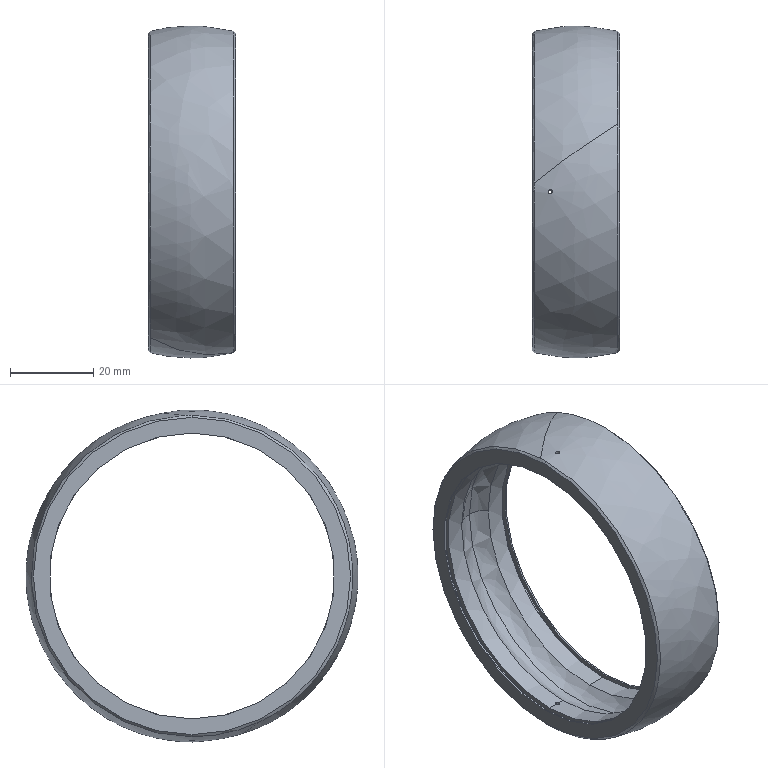Part | SolidWorks | features BaseBody 1 | 1 solid | 32 faces | box 21 x 80 x 80 mm | volume 21730 mm3 | spline 26 | plane 6
STEP:
#1=CARTESIAN_POINT('',(0.,111.35,49.2));
#2=VERTEX_POINT('',#1);
#3=CARTESIAN_POINT('',(0.,38.65,49.2));
#4=VERTEX_POINT('',#3);
#5=CARTESIAN_POINT('',(0.,75.,49.2));
#6=DIRECTION('',(-1.,0.,0.));
#7=DIRECTION('',(0.,-1.,0.));
#8=AXIS2_PLACEMENT_3D('',#5,#6,#7);
#9=CIRCLE('',#8,36.35);
#10=EDGE_CURVE('',#2,#4,#9,.T.);
#11=ORIENTED_EDGE('',*,*,#10,.F.);
#12=CARTESIAN_POINT('',(-4.535,109.445,49.2));
#13=VERTEX_POINT('',#12);
#14=CARTESIAN_POINT('',(0.,105.,49.2));
#15=DIRECTION('',(0.,0.,1.));
#16=DIRECTION('',(0.,1.,0.));
#17=AXIS2_PLACEMENT_3D('',#14,#15,#16);
#18=CIRCLE('',#17,6.35);
#19=EDGE_CURVE('',#2,#13,#18,.T.);
#20=ORIENTED_EDGE('',*,*,#19,.T.);
#21=CARTESIAN_POINT('',(-4.535,75.,14.755));
#22=VERTEX_POINT('',#21);
#23=CARTESIAN_POINT('',(-4.535,75.,49.2));
#24=DIRECTION('',(-1.,0.,0.));
#25=DIRECTION('',(0.,0.,1.));
#26=AXIS2_PLACEMENT_3D('',#23,#24,#25);
#27=CIRCLE('',#26,34.445);
#28=EDGE_CURVE('',#13,#22,#27,.T.);
#29=ORIENTED_EDGE('',*,*,#28,.T.);
#30=CARTESIAN_POINT('',(-4.535,40.555,49.2));
#31=VERTEX_POINT('',#30);
#32=CARTESIAN_POINT('',(-4.535,75.,49.2));
#33=DIRECTION('',(-1.,0.,0.));
#34=DIRECTION('',(0.,0.,1.));
#35=AXIS2_PLACEMENT_3D('',#32,#33,#34);
#36=CIRCLE('',#35,34.445);
#37=EDGE_CURVE('',#22,#31,#36,.T.);
#38=ORIENTED_EDGE('',*,*,#37,.T.);
#39=CARTESIAN_POINT('',(0.,45.,49.2));
#40=DIRECTION('',(0.,0.,-1.));
#41=DIRECTION('',(0.,-1.,0.));
#42=AXIS2_PLACEMENT_3D('',#39,#40,#41);
#43=CIRCLE('',#42,6.35);
#44=EDGE_CURVE('',#4,#31,#43,.T.);
#45=ORIENTED_EDGE('',*,*,#44,.F.);
#46=EDGE_LOOP('',(#11,#20,#29,#38,#45));
#47=FACE_OUTER_BOUND('',#46,.T.);
#48=CARTESIAN_POINT('',(0.,111.35,49.2));
#49=CARTESIAN_POINT('',(0.,111.35,-23.5));
#50=CARTESIAN_POINT('',(0.,38.65,-23.5));
#51=CARTESIAN_POINT('',(0.,38.65,49.2));
#52=CARTESIAN_POINT('',(-1.73,111.35,49.2));
#53=CARTESIAN_POINT('',(-1.73,111.35,-23.5));
#54=CARTESIAN_POINT('',(-1.73,38.65,-23.5));
#55=CARTESIAN_POINT('',(-1.73,38.65,49.2));
#56=CARTESIAN_POINT('',(-3.324,110.68,49.2));
#57=CARTESIAN_POINT('',(-3.324,110.68,-22.16));
#58=CARTESIAN_POINT('',(-3.324,39.32,-22.16));
#59=CARTESIAN_POINT('',(-3.324,39.32,49.2));
#60=CARTESIAN_POINT('',(-4.535,109.445,49.2));
#61=CARTESIAN_POINT('',(-4.535,109.445,-19.69));
#62=CARTESIAN_POINT('',(-4.535,40.555,-19.69));
#63=CARTESIAN_POINT('',(-4.535,40.555,49.2));
#64=(BOUNDED_SURFACE()B_SPLINE_SURFACE(3,3,((#48,#49,#50,#51),(#52,#53,#54,#55),(#56,#57,#58,#59),(#60,#61,#62,#63)),.UNSPECIFIED.,.F.,.F.,.F.)B_SPLINE_SURFACE_WITH_KNOTS((4,4),(4,4),(0.,1.),(0.,1.),.UNSPECIFIED.)GEOMETRIC_REPRESENTATION_ITEM()RATIONAL_B_SPLINE_SURFACE(((1.,0.3333,0.3333,1.),(0.948,0.316,0.316,0.948),(0.948,0.316,0.316,0.948),(1.,0.3333,0.3333,1.)))REPRESENTATION_ITEM('')SURFACE());
#65=ADVANCED_FACE('',(#47),#64,.T.);
#66=CARTESIAN_POINT('',(10.,75.,10.47));
#67=VERTEX_POINT('',#66);
#68=CARTESIAN_POINT('',(10.,72.909,10.527));
#69=VERTEX_POINT('',#68);
#70=CARTESIAN_POINT('',(10.,75.,49.2));
#71=DIRECTION('',(-1.,0.,0.));
#72=DIRECTION('',(0.,0.,1.));
#73=AXIS2_PLACEMENT_3D('',#70,#71,#72);
#74=CIRCLE('',#73,38.73);
#75=EDGE_CURVE('',#67,#69,#74,.T.);
#76=ORIENTED_EDGE('',*,*,#75,.F.);
#77=CARTESIAN_POINT('',(10.5,75.,10.97));
#78=VERTEX_POINT('',#77);
#79=CARTESIAN_POINT('',(10.25,75.,10.72));
#80=DIRECTION('',(0.7071,0.,0.7071));
#81=VECTOR('',#80,1000.);
#82=LINE('',#79,#81);
#83=EDGE_CURVE('',#67,#78,#82,.T.);
#84=ORIENTED_EDGE('',*,*,#83,.T.);
#85=CARTESIAN_POINT('',(10.5,75.,87.43));
#86=VERTEX_POINT('',#85);
#87=CARTESIAN_POINT('',(10.5,75.,49.2));
#88=DIRECTION('',(-1.,0.,0.));
#89=DIRECTION('',(0.,0.,1.));
#90=AXIS2_PLACEMENT_3D('',#87,#88,#89);
#91=CIRCLE('',#90,38.23);
#92=EDGE_CURVE('',#78,#86,#91,.T.);
#93=ORIENTED_EDGE('',*,*,#92,.T.);
#94=CARTESIAN_POINT('',(10.,75.,87.93));
#95=VERTEX_POINT('',#94);
#96=CARTESIAN_POINT('',(10.25,75.,87.68));
#97=DIRECTION('',(0.7071,0.,-0.7071));
#98=VECTOR('',#97,1000.);
#99=LINE('',#96,#98);
#100=EDGE_CURVE('',#95,#86,#99,.T.);
#101=ORIENTED_EDGE('',*,*,#100,.F.);
#102=CARTESIAN_POINT('',(10.,75.,49.2));
#103=DIRECTION('',(-1.,0.,0.));
#104=DIRECTION('',(0.,0.,1.));
#105=AXIS2_PLACEMENT_3D('',#102,#103,#104);
#106=CIRCLE('',#105,38.73);
#107=EDGE_CURVE('',#69,#95,#106,.T.);
#108=ORIENTED_EDGE('',*,*,#107,.F.);
#109=EDGE_LOOP('',(#76,#84,#93,#101,#108));
#110=FACE_OUTER_BOUND('',#109,.T.);
#111=CARTESIAN_POINT('',(10.,75.,10.47));
#112=CARTESIAN_POINT('',(10.,-2.46,10.47));
#113=CARTESIAN_POINT('',(10.,-2.46,87.93));
#114=CARTESIAN_POINT('',(10.,75.,87.93));
#115=CARTESIAN_POINT('',(10.5,75.,10.97));
#116=CARTESIAN_POINT('',(10.5,-1.46,10.97));
#117=CARTESIAN_POINT('',(10.5,-1.46,87.43));
#118=CARTESIAN_POINT('',(10.5,75.,87.43));
#119=(BOUNDED_SURFACE()B_SPLINE_SURFACE(1,3,((#111,#112,#113,#114),(#115,#116,#117,#118)),.UNSPECIFIED.,.F.,.F.,.F.)B_SPLINE_SURFACE_WITH_KNOTS((2,2),(4,4),(0.,1.),(0.,1.),.UNSPECIFIED.)GEOMETRIC_REPRESENTATION_ITEM()RATIONAL_B_SPLINE_SURFACE(((1.,0.3333,0.3333,1.),(1.,0.3333,0.3333,1.)))REPRESENTATION_ITEM('')SURFACE());
#120=ADVANCED_FACE('',(#110),#119,.T.);
#121=CARTESIAN_POINT('',(-5.7,75.,9.608));
#122=VERTEX_POINT('',#121);
#123=CARTESIAN_POINT('',(-6.7,75.,9.765));
#124=VERTEX_POINT('',#123);
#125=CARTESIAN_POINT('',(-5.7,75.,9.608));
#126=CARTESIAN_POINT('',(-5.7,75.133,9.608));
#127=CARTESIAN_POINT('',(-5.755,75.263,9.617));
#128=CARTESIAN_POINT('',(-5.94,75.447,9.646));
#129=CARTESIAN_POINT('',(-6.07,75.5,9.666));
#130=CARTESIAN_POINT('',(-6.329,75.5,9.707));
#131=CARTESIAN_POINT('',(-6.459,75.448,9.727));
#132=CARTESIAN_POINT('',(-6.646,75.262,9.757));
#133=CARTESIAN_POINT('',(-6.7,75.133,9.765));
#134=CARTESIAN_POINT('',(-6.7,75.,9.765));
#135=B_SPLINE_CURVE_WITH_KNOTS('',3,(#125,#126,#127,#128,#129,#130,#131,#132,#133,#134),.UNSPECIFIED.,.F.,.F.,(4,2,2,2,4),(0.001573,0.001966,0.002359,0.002752,0.003145),.UNSPECIFIED.);
#136=EDGE_CURVE('',#122,#124,#135,.T.);
#137=ORIENTED_EDGE('',*,*,#136,.T.);
#138=CARTESIAN_POINT('',(-6.7,75.,9.765));
#139=CARTESIAN_POINT('',(-6.7,74.867,9.765));
#140=CARTESIAN_POINT('',(-6.645,74.737,9.756));
#141=CARTESIAN_POINT('',(-6.46,74.553,9.727));
#142=CARTESIAN_POINT('',(-6.33,74.5,9.707));
#143=CARTESIAN_POINT('',(-6.071,74.5,9.666));
#144=CARTESIAN_POINT('',(-5.941,74.552,9.646));
#145=CARTESIAN_POINT('',(-5.754,74.738,9.617));
#146=CARTESIAN_POINT('',(-5.7,74.867,9.608));
#147=CARTESIAN_POINT('',(-5.7,75.,9.608));
#148=B_SPLINE_CURVE_WITH_KNOTS('',3,(#138,#139,#140,#141,#142,#143,#144,#145,#146,#147),.UNSPECIFIED.,.F.,.F.,(4,2,2,2,4),(0.,0.0003932,0.0007863,0.001179,0.001573),.UNSPECIFIED.);
#149=EDGE_CURVE('',#124,#122,#148,.T.);
#150=ORIENTED_EDGE('',*,*,#149,.T.);
#151=EDGE_LOOP('',(#137,#150));
#152=FACE_BOUND('',#151,.T.);
#153=CARTESIAN_POINT('',(10.,91.345,84.312));
#154=VERTEX_POINT('',#153);
#155=CARTESIAN_POINT('',(10.,75.,49.2));
#156=DIRECTION('',(-1.,0.,0.));
#157=DIRECTION('',(0.,0.,1.));
#158=AXIS2_PLACEMENT_3D('',#155,#156,#157);
#159=CIRCLE('',#158,38.73);
#160=EDGE_CURVE('',#154,#67,#159,.T.);
#161=ORIENTED_EDGE('',*,*,#160,.T.);
#162=ORIENTED_EDGE('',*,*,#75,.T.);
#163=CARTESIAN_POINT('',(-10.,58.655,14.088));
#164=VERTEX_POINT('',#163);
#165=CARTESIAN_POINT('',(0.,75.,49.2));
#166=DIRECTION('',(-0.592,0.7819,-0.1954));
#167=DIRECTION('',(0.7421,0.6234,0.2461));
#168=AXIS2_PLACEMENT_3D('',#165,#166,#167);
#169=CIRCLE('',#168,40.);
#170=EDGE_CURVE('',#69,#164,#169,.T.);
#171=ORIENTED_EDGE('',*,*,#170,.T.);
#172=CARTESIAN_POINT('',(-10.,75.,10.47));
#173=VERTEX_POINT('',#172);
#174=CARTESIAN_POINT('',(-10.,75.,49.2));
#175=DIRECTION('',(-1.,0.,0.));
#176=DIRECTION('',(0.,0.,1.));
#177=AXIS2_PLACEMENT_3D('',#174,#175,#176);
#178=CIRCLE('',#177,38.73);
#179=EDGE_CURVE('',#173,#164,#178,.T.);
#180=ORIENTED_EDGE('',*,*,#179,.F.);
#181=CARTESIAN_POINT('',(-10.,77.091,87.873));
#182=VERTEX_POINT('',#181);
#183=CARTESIAN_POINT('',(-10.,75.,49.2));
#184=DIRECTION('',(-1.,0.,0.));
#185=DIRECTION('',(0.,0.,1.));
#186=AXIS2_PLACEMENT_3D('',#183,#184,#185);
#187=CIRCLE('',#186,38.73);
#188=EDGE_CURVE('',#182,#173,#187,.T.);
#189=ORIENTED_EDGE('',*,*,#188,.F.);
#190=CARTESIAN_POINT('',(0.,75.,49.2));
#191=DIRECTION('',(0.592,-0.7819,0.1954));
#192=DIRECTION('',(0.7421,0.6234,0.2461));
#193=AXIS2_PLACEMENT_3D('',#190,#191,#192);
#194=CIRCLE('',#193,40.);
#195=EDGE_CURVE('',#154,#182,#194,.T.);
#196=ORIENTED_EDGE('',*,*,#195,.F.);
#197=EDGE_LOOP('',(#161,#162,#171,#180,#189,#196));
#198=FACE_OUTER_BOUND('',#197,.T.);
#199=CARTESIAN_POINT('',(31.786,96.038,37.074));
#200=CARTESIAN_POINT('',(6.311,129.683,28.667));
#201=CARTESIAN_POINT('',(-7.211,129.652,69.518));
#202=CARTESIAN_POINT('',(18.264,96.007,77.925));
#203=CARTESIAN_POINT('',(28.23,87.172,12.371));
#204=CARTESIAN_POINT('',(-23.683,155.733,-4.76));
#205=CARTESIAN_POINT('',(-51.237,155.67,78.484));
#206=CARTESIAN_POINT('',(0.6755,87.109,95.615));
#207=CARTESIAN_POINT('',(9.909,70.821,2.447));
#208=CARTESIAN_POINT('',(-46.327,145.093,-16.111));
#209=CARTESIAN_POINT('',(-76.176,145.024,74.068));
#210=CARTESIAN_POINT('',(-19.94,70.753,92.626));
#211=CARTESIAN_POINT('',(-10.314,58.463,14.269));
#212=CARTESIAN_POINT('',(-45.726,105.232,2.583));
#213=CARTESIAN_POINT('',(-64.523,105.189,59.37));
#214=CARTESIAN_POINT('',(-29.11,58.42,71.056));
#215=(BOUNDED_SURFACE()B_SPLINE_SURFACE(3,3,((#199,#200,#201,#202),(#203,#204,#205,#206),(#207,#208,#209,#210),(#211,#212,#213,#214)),.UNSPECIFIED.,.F.,.F.,.F.)B_SPLINE_SURFACE_WITH_KNOTS((4,4),(4,4),(0.,1.),(0.,1.),.UNSPECIFIED.)GEOMETRIC_REPRESENTATION_ITEM()RATIONAL_B_SPLINE_SURFACE(((1.,0.3333,0.3333,1.),(0.766,0.2553,0.2553,0.766),(0.766,0.2553,0.2553,0.766),(1.,0.3333,0.3333,1.)))REPRESENTATION_ITEM('')SURFACE());
#216=ADVANCED_FACE('',(#152,#198),#215,.T.);
#217=CARTESIAN_POINT('',(-10.,75.,87.93));
#218=VERTEX_POINT('',#217);
#219=CARTESIAN_POINT('',(-10.,75.,49.2));
#220=DIRECTION('',(-1.,0.,0.));
#221=DIRECTION('',(0.,0.,1.));
#222=AXIS2_PLACEMENT_3D('',#219,#220,#221);
#223=CIRCLE('',#222,38.73);
#224=EDGE_CURVE('',#218,#182,#223,.T.);
#225=ORIENTED_EDGE('',*,*,#224,.T.);
#226=ORIENTED_EDGE('',*,*,#188,.T.);
#227=CARTESIAN_POINT('',(-10.5,75.,10.97));
#228=VERTEX_POINT('',#227);
#229=CARTESIAN_POINT('',(-10.25,75.,10.72));
#230=DIRECTION('',(-0.7071,0.,0.7071));
#231=VECTOR('',#230,1000.);
#232=LINE('',#229,#231);
#233=EDGE_CURVE('',#173,#228,#232,.T.);
#234=ORIENTED_EDGE('',*,*,#233,.T.);
#235=CARTESIAN_POINT('',(-10.5,75.,87.43));
#236=VERTEX_POINT('',#235);
#237=CARTESIAN_POINT('',(-10.5,75.,49.2));
#238=DIRECTION('',(-1.,0.,0.));
#239=DIRECTION('',(0.,0.,1.));
#240=AXIS2_PLACEMENT_3D('',#237,#238,#239);
#241=CIRCLE('',#240,38.23);
#242=EDGE_CURVE('',#236,#228,#241,.T.);
#243=ORIENTED_EDGE('',*,*,#242,.F.);
#244=CARTESIAN_POINT('',(-10.25,75.,87.68));
#245=DIRECTION('',(-0.7071,0.,-0.7071));
#246=VECTOR('',#245,1000.);
#247=LINE('',#244,#246);
#248=EDGE_CURVE('',#218,#236,#247,.T.);
#249=ORIENTED_EDGE('',*,*,#248,.F.);
#250=EDGE_LOOP('',(#225,#226,#234,#243,#249));
#251=FACE_OUTER_BOUND('',#250,.T.);
#252=CARTESIAN_POINT('',(-10.,75.,10.47));
#253=CARTESIAN_POINT('',(-10.,152.46,10.47));
#254=CARTESIAN_POINT('',(-10.,152.46,87.93));
#255=CARTESIAN_POINT('',(-10.,75.,87.93));
#256=CARTESIAN_POINT('',(-10.5,75.,10.97));
#257=CARTESIAN_POINT('',(-10.5,151.46,10.97));
#258=CARTESIAN_POINT('',(-10.5,151.46,87.43));
#259=CARTESIAN_POINT('',(-10.5,75.,87.43));
#260=(BOUNDED_SURFACE()B_SPLINE_SURFACE(1,3,((#252,#253,#254,#255),(#256,#257,#258,#259)),.UNSPECIFIED.,.F.,.F.,.F.)B_SPLINE_SURFACE_WITH_KNOTS((2,2),(4,4),(0.,1.),(0.,1.),.UNSPECIFIED.)GEOMETRIC_REPRESENTATION_ITEM()RATIONAL_B_SPLINE_SURFACE(((1.,0.3333,0.3333,1.),(1.,0.3333,0.3333,1.)))REPRESENTATION_ITEM('')SURFACE());
#261=ADVANCED_FACE('',(#251),#260,.T.);
#262=CARTESIAN_POINT('',(4.535,109.445,49.2));
#263=VERTEX_POINT('',#262);
#264=CARTESIAN_POINT('',(4.535,75.,14.755));
#265=VERTEX_POINT('',#264);
#266=CARTESIAN_POINT('',(4.535,75.,49.2));
#267=DIRECTION('',(-1.,0.,0.));
#268=DIRECTION('',(0.,0.,1.));
#269=AXIS2_PLACEMENT_3D('',#266,#267,#268);
#270=CIRCLE('',#269,34.445);
#271=EDGE_CURVE('',#263,#265,#270,.T.);
#272=ORIENTED_EDGE('',*,*,#271,.F.);
#273=CARTESIAN_POINT('',(0.,105.,49.2));
#274=DIRECTION('',(0.,0.,1.));
#275=DIRECTION('',(0.,1.,0.));
#276=AXIS2_PLACEMENT_3D('',#273,#274,#275);
#277=CIRCLE('',#276,6.35);
#278=EDGE_CURVE('',#263,#2,#277,.T.);
#279=ORIENTED_EDGE('',*,*,#278,.T.);
#280=ORIENTED_EDGE('',*,*,#10,.T.);
#281=CARTESIAN_POINT('',(4.535,40.555,49.2));
#282=VERTEX_POINT('',#281);
#283=CARTESIAN_POINT('',(0.,45.,49.2));
#284=DIRECTION('',(0.,0.,-1.));
#285=DIRECTION('',(0.,-1.,0.));
#286=AXIS2_PLACEMENT_3D('',#283,#284,#285);
#287=CIRCLE('',#286,6.35);
#288=EDGE_CURVE('',#282,#4,#287,.T.);
#289=ORIENTED_EDGE('',*,*,#288,.F.);
#290=CARTESIAN_POINT('',(4.535,75.,49.2));
#291=DIRECTION('',(-1.,0.,0.));
#292=DIRECTION('',(0.,0.,1.));
#293=AXIS2_PLACEMENT_3D('',#290,#291,#292);
#294=CIRCLE('',#293,34.445);
#295=EDGE_CURVE('',#265,#282,#294,.T.);
#296=ORIENTED_EDGE('',*,*,#295,.F.);
#297=EDGE_LOOP('',(#272,#279,#280,#289,#296));
#298=FACE_OUTER_BOUND('',#297,.T.);
#299=CARTESIAN_POINT('',(4.535,109.445,49.2));
#300=CARTESIAN_POINT('',(4.535,109.445,-19.69));
#301=CARTESIAN_POINT('',(4.535,40.555,-19.69));
#302=CARTESIAN_POINT('',(4.535,40.555,49.2));
#303=CARTESIAN_POINT('',(3.324,110.68,49.2));
#304=CARTESIAN_POINT('',(3.324,110.68,-22.16));
#305=CARTESIAN_POINT('',(3.324,39.32,-22.16));
#306=CARTESIAN_POINT('',(3.324,39.32,49.2));
#307=CARTESIAN_POINT('',(1.73,111.35,49.2));
#308=CARTESIAN_POINT('',(1.73,111.35,-23.5));
#309=CARTESIAN_POINT('',(1.73,38.65,-23.5));
#310=CARTESIAN_POINT('',(1.73,38.65,49.2));
#311=CARTESIAN_POINT('',(0.,111.35,49.2));
#312=CARTESIAN_POINT('',(0.,111.35,-23.5));
#313=CARTESIAN_POINT('',(0.,38.65,-23.5));
#314=CARTESIAN_POINT('',(0.,38.65,49.2));
#315=(BOUNDED_SURFACE()B_SPLINE_SURFACE(3,3,((#299,#300,#301,#302),(#303,#304,#305,#306),(#307,#308,#309,#310),(#311,#312,#313,#314)),.UNSPECIFIED.,.F.,.F.,.F.)B_SPLINE_SURFACE_WITH_KNOTS((4,4),(4,4),(0.,1.),(0.,1.),.UNSPECIFIED.)GEOMETRIC_REPRESENTATION_ITEM()RATIONAL_B_SPLINE_SURFACE(((1.,0.3333,0.3333,1.),(0.948,0.316,0.316,0.948),(0.948,0.316,0.316,0.948),(1.,0.3333,0.3333,1.)))REPRESENTATION_ITEM('')SURFACE());
#316=ADVANCED_FACE('',(#298),#315,.T.);
#317=CARTESIAN_POINT('',(-6.7,75.,83.645));
#318=VERTEX_POINT('',#317);
#319=CARTESIAN_POINT('',(-5.7,75.,83.645));
#320=VERTEX_POINT('',#319);
#321=CARTESIAN_POINT('',(-6.7,75.,83.645));
#322=CARTESIAN_POINT('',(-6.7,74.868,83.645));
#323=CARTESIAN_POINT('',(-6.646,74.739,83.644));
#324=CARTESIAN_POINT('',(-6.462,74.554,83.642));
#325=CARTESIAN_POINT('',(-6.332,74.5,83.641));
#326=CARTESIAN_POINT('',(-6.068,74.5,83.641));
#327=CARTESIAN_POINT('',(-5.939,74.554,83.642));
#328=CARTESIAN_POINT('',(-5.754,74.738,83.644));
#329=CARTESIAN_POINT('',(-5.7,74.868,83.645));
#330=CARTESIAN_POINT('',(-5.7,75.,83.645));
#331=B_SPLINE_CURVE_WITH_KNOTS('',3,(#321,#322,#323,#324,#325,#326,#327,#328,#329,#330),.UNSPECIFIED.,.F.,.F.,(4,2,2,2,4),(0.001562,0.001953,0.002343,0.002734,0.003124),.UNSPECIFIED.);
#332=EDGE_CURVE('',#318,#320,#331,.T.);
#333=ORIENTED_EDGE('',*,*,#332,.F.);
#334=CARTESIAN_POINT('',(-6.7,75.,88.635));
#335=VERTEX_POINT('',#334);
#336=CARTESIAN_POINT('',(-6.7,75.,86.421));
#337=DIRECTION('',(0.,0.,1.));
#338=VECTOR('',#337,1000.);
#339=LINE('',#336,#338);
#340=EDGE_CURVE('',#318,#335,#339,.T.);
#341=ORIENTED_EDGE('',*,*,#340,.T.);
#342=CARTESIAN_POINT('',(-5.7,75.,88.792));
#343=VERTEX_POINT('',#342);
#344=CARTESIAN_POINT('',(-5.7,75.,88.792));
#345=CARTESIAN_POINT('',(-5.7,74.867,88.792));
#346=CARTESIAN_POINT('',(-5.755,74.737,88.783));
#347=CARTESIAN_POINT('',(-5.94,74.553,88.754));
#348=CARTESIAN_POINT('',(-6.07,74.5,88.734));
#349=CARTESIAN_POINT('',(-6.329,74.5,88.693));
#350=CARTESIAN_POINT('',(-6.459,74.552,88.673));
#351=CARTESIAN_POINT('',(-6.646,74.738,88.643));
#352=CARTESIAN_POINT('',(-6.7,74.867,88.635));
#353=CARTESIAN_POINT('',(-6.7,75.,88.635));
#354=B_SPLINE_CURVE_WITH_KNOTS('',3,(#344,#345,#346,#347,#348,#349,#350,#351,#352,#353),.UNSPECIFIED.,.F.,.F.,(4,2,2,2,4),(0.001573,0.001966,0.002359,0.002752,0.003145),.UNSPECIFIED.);
#355=EDGE_CURVE('',#343,#335,#354,.T.);
#356=ORIENTED_EDGE('',*,*,#355,.F.);
#357=CARTESIAN_POINT('',(-5.7,75.,86.421));
#358=DIRECTION('',(0.,0.,1.));
#359=VECTOR('',#358,1000.);
#360=LINE('',#357,#359);
#361=EDGE_CURVE('',#320,#343,#360,.T.);
#362=ORIENTED_EDGE('',*,*,#361,.F.);
#363=EDGE_LOOP('',(#333,#341,#356,#362));
#364=FACE_OUTER_BOUND('',#363,.T.);
#365=CARTESIAN_POINT('',(-5.7,75.,83.61));
#366=CARTESIAN_POINT('',(-5.7,75.,88.823));
#367=CARTESIAN_POINT('',(-5.7,74.,83.61));
#368=CARTESIAN_POINT('',(-5.7,74.,88.823));
#369=CARTESIAN_POINT('',(-6.7,74.,83.61));
#370=CARTESIAN_POINT('',(-6.7,74.,88.823));
#371=CARTESIAN_POINT('',(-6.7,75.,83.61));
#372=CARTESIAN_POINT('',(-6.7,75.,88.823));
#373=(BOUNDED_SURFACE()B_SPLINE_SURFACE(3,1,((#365,#366),(#367,#368),(#369,#370),(#371,#372)),.UNSPECIFIED.,.F.,.F.,.F.)B_SPLINE_SURFACE_WITH_KNOTS((4,4),(2,2),(0.,1.),(0.,1.),.UNSPECIFIED.)GEOMETRIC_REPRESENTATION_ITEM()RATIONAL_B_SPLINE_SURFACE(((1.,1.),(0.3333,0.3333),(0.3333,0.3333),(1.,1.)))REPRESENTATION_ITEM('')SURFACE());
#374=ADVANCED_FACE('',(#364),#373,.T.);
#375=ORIENTED_EDGE('',*,*,#149,.F.);
#376=CARTESIAN_POINT('',(-6.7,75.,14.755));
#377=VERTEX_POINT('',#376);
#378=CARTESIAN_POINT('',(-6.7,75.,11.979));
#379=DIRECTION('',(0.,0.,1.));
#380=VECTOR('',#379,1000.);
#381=LINE('',#378,#380);
#382=EDGE_CURVE('',#124,#377,#381,.T.);
#383=ORIENTED_EDGE('',*,*,#382,.T.);
#384=CARTESIAN_POINT('',(-5.7,75.,14.755));
#385=VERTEX_POINT('',#384);
#386=CARTESIAN_POINT('',(-5.7,75.,14.755));
#387=CARTESIAN_POINT('',(-5.7,74.868,14.755));
#388=CARTESIAN_POINT('',(-5.754,74.739,14.756));
#389=CARTESIAN_POINT('',(-5.938,74.554,14.758));
#390=CARTESIAN_POINT('',(-6.068,74.5,14.759));
#391=CARTESIAN_POINT('',(-6.332,74.5,14.759));
#392=CARTESIAN_POINT('',(-6.461,74.554,14.758));
#393=CARTESIAN_POINT('',(-6.646,74.738,14.756));
#394=CARTESIAN_POINT('',(-6.7,74.868,14.755));
#395=CARTESIAN_POINT('',(-6.7,75.,14.755));
#396=B_SPLINE_CURVE_WITH_KNOTS('',3,(#386,#387,#388,#389,#390,#391,#392,#393,#394,#395),.UNSPECIFIED.,.F.,.F.,(4,2,2,2,4),(0.001562,0.001953,0.002343,0.002734,0.003124),.UNSPECIFIED.);
#397=EDGE_CURVE('',#385,#377,#396,.T.);
#398=ORIENTED_EDGE('',*,*,#397,.F.);
#399=CARTESIAN_POINT('',(-5.7,75.,11.979));
#400=DIRECTION('',(0.,0.,1.));
#401=VECTOR('',#400,1000.);
#402=LINE('',#399,#401);
#403=EDGE_CURVE('',#122,#385,#402,.T.);
#404=ORIENTED_EDGE('',*,*,#403,.F.);
#405=EDGE_LOOP('',(#375,#383,#398,#404));
#406=FACE_OUTER_BOUND('',#405,.T.);
#407=CARTESIAN_POINT('',(-5.7,75.,9.577));
#408=CARTESIAN_POINT('',(-5.7,75.,14.79));
#409=CARTESIAN_POINT('',(-5.7,74.,9.577));
#410=CARTESIAN_POINT('',(-5.7,74.,14.79));
#411=CARTESIAN_POINT('',(-6.7,74.,9.577));
#412=CARTESIAN_POINT('',(-6.7,74.,14.79));
#413=CARTESIAN_POINT('',(-6.7,75.,9.577));
#414=CARTESIAN_POINT('',(-6.7,75.,14.79));
#415=(BOUNDED_SURFACE()B_SPLINE_SURFACE(3,1,((#407,#408),(#409,#410),(#411,#412),(#413,#414)),.UNSPECIFIED.,.F.,.F.,.F.)B_SPLINE_SURFACE_WITH_KNOTS((4,4),(2,2),(0.,1.),(0.,1.),.UNSPECIFIED.)GEOMETRIC_REPRESENTATION_ITEM()RATIONAL_B_SPLINE_SURFACE(((1.,1.),(0.3333,0.3333),(0.3333,0.3333),(1.,1.)))REPRESENTATION_ITEM('')SURFACE());
#416=ADVANCED_FACE('',(#406),#415,.T.);
#417=CARTESIAN_POINT('',(-10.1,75.,14.755));
#418=VERTEX_POINT('',#417);
#419=CARTESIAN_POINT('',(-10.1,75.,83.645));
#420=VERTEX_POINT('',#419);
#421=CARTESIAN_POINT('',(-10.1,75.,49.2));
#422=DIRECTION('',(-1.,0.,0.));
#423=DIRECTION('',(0.,0.,1.));
#424=AXIS2_PLACEMENT_3D('',#421,#422,#423);
#425=CIRCLE('',#424,34.445);
#426=EDGE_CURVE('',#418,#420,#425,.T.);
#427=ORIENTED_EDGE('',*,*,#426,.F.);
#428=CARTESIAN_POINT('',(-10.5,75.,14.755));
#429=VERTEX_POINT('',#428);
#430=CARTESIAN_POINT('',(-10.3,75.,14.755));
#431=DIRECTION('',(-1.,0.,0.));
#432=VECTOR('',#431,1000.);
#433=LINE('',#430,#432);
#434=EDGE_CURVE('',#418,#429,#433,.T.);
#435=ORIENTED_EDGE('',*,*,#434,.T.);
#436=CARTESIAN_POINT('',(-10.5,75.,83.645));
#437=VERTEX_POINT('',#436);
#438=CARTESIAN_POINT('',(-10.5,75.,49.2));
#439=DIRECTION('',(-1.,0.,0.));
#440=DIRECTION('',(0.,0.,1.));
#441=AXIS2_PLACEMENT_3D('',#438,#439,#440);
#442=CIRCLE('',#441,34.445);
#443=EDGE_CURVE('',#429,#437,#442,.T.);
#444=ORIENTED_EDGE('',*,*,#443,.T.);
#445=CARTESIAN_POINT('',(-10.3,75.,83.645));
#446=DIRECTION('',(-1.,0.,0.));
#447=VECTOR('',#446,1000.);
#448=LINE('',#445,#447);
#449=EDGE_CURVE('',#420,#437,#448,.T.);
#450=ORIENTED_EDGE('',*,*,#449,.F.);
#451=EDGE_LOOP('',(#427,#435,#444,#450));
#452=FACE_OUTER_BOUND('',#451,.T.);
#453=CARTESIAN_POINT('',(-10.1,75.,83.645));
#454=CARTESIAN_POINT('',(-10.5,75.,83.645));
#455=CARTESIAN_POINT('',(-10.1,6.11,83.645));
#456=CARTESIAN_POINT('',(-10.5,6.11,83.645));
#457=CARTESIAN_POINT('',(-10.1,6.11,14.755));
#458=CARTESIAN_POINT('',(-10.5,6.11,14.755));
#459=CARTESIAN_POINT('',(-10.1,75.,14.755));
#460=CARTESIAN_POINT('',(-10.5,75.,14.755));
#461=(BOUNDED_SURFACE()B_SPLINE_SURFACE(3,1,((#453,#454),(#455,#456),(#457,#458),(#459,#460)),.UNSPECIFIED.,.F.,.F.,.F.)B_SPLINE_SURFACE_WITH_KNOTS((4,4),(2,2),(0.,1.),(0.,1.),.UNSPECIFIED.)GEOMETRIC_REPRESENTATION_ITEM()RATIONAL_B_SPLINE_SURFACE(((1.,1.),(0.3333,0.3333),(0.3333,0.3333),(1.,1.)))REPRESENTATION_ITEM('')SURFACE());
#462=ADVANCED_FACE('',(#452),#461,.T.);
#463=CARTESIAN_POINT('',(-9.1,75.,13.755));
#464=VERTEX_POINT('',#463);
#465=CARTESIAN_POINT('',(-9.1,75.,84.645));
#466=VERTEX_POINT('',#465);
#467=CARTESIAN_POINT('',(-9.1,75.,49.2));
#468=DIRECTION('',(-1.,0.,0.));
#469=DIRECTION('',(0.,0.,1.));
#470=AXIS2_PLACEMENT_3D('',#467,#468,#469);
#471=CIRCLE('',#470,35.445);
#472=EDGE_CURVE('',#464,#466,#471,.T.);
#473=ORIENTED_EDGE('',*,*,#472,.F.);
#474=CARTESIAN_POINT('',(-10.1,75.,13.755));
#475=VERTEX_POINT('',#474);
#476=CARTESIAN_POINT('',(-9.6,75.,13.755));
#477=DIRECTION('',(-1.,0.,0.));
#478=VECTOR('',#477,1000.);
#479=LINE('',#476,#478);
#480=EDGE_CURVE('',#464,#475,#479,.T.);
#481=ORIENTED_EDGE('',*,*,#480,.T.);
#482=CARTESIAN_POINT('',(-10.1,75.,84.645));
#483=VERTEX_POINT('',#482);
#484=CARTESIAN_POINT('',(-10.1,75.,49.2));
#485=DIRECTION('',(-1.,0.,0.));
#486=DIRECTION('',(0.,0.,1.));
#487=AXIS2_PLACEMENT_3D('',#484,#485,#486);
#488=CIRCLE('',#487,35.445);
#489=EDGE_CURVE('',#475,#483,#488,.T.);
#490=ORIENTED_EDGE('',*,*,#489,.T.);
#491=CARTESIAN_POINT('',(-9.6,75.,84.645));
#492=DIRECTION('',(-1.,0.,0.));
#493=VECTOR('',#492,1000.);
#494=LINE('',#491,#493);
#495=EDGE_CURVE('',#466,#483,#494,.T.);
#496=ORIENTED_EDGE('',*,*,#495,.F.);
#497=EDGE_LOOP('',(#473,#481,#490,#496));
#498=FACE_OUTER_BOUND('',#497,.T.);
#499=CARTESIAN_POINT('',(-9.1,75.,84.645));
#500=CARTESIAN_POINT('',(-10.1,75.,84.645));
#501=CARTESIAN_POINT('',(-9.1,4.11,84.645));
#502=CARTESIAN_POINT('',(-10.1,4.11,84.645));
#503=CARTESIAN_POINT('',(-9.1,4.11,13.755));
#504=CARTESIAN_POINT('',(-10.1,4.11,13.755));
#505=CARTESIAN_POINT('',(-9.1,75.,13.755));
#506=CARTESIAN_POINT('',(-10.1,75.,13.755));
#507=(BOUNDED_SURFACE()B_SPLINE_SURFACE(3,1,((#499,#500),(#501,#502),(#503,#504),(#505,#506)),.UNSPECIFIED.,.F.,.F.,.T.)B_SPLINE_SURFACE_WITH_KNOTS((4,4),(2,2),(0.,1.),(0.,1.),.UNSPECIFIED.)GEOMETRIC_REPRESENTATION_ITEM()RATIONAL_B_SPLINE_SURFACE(((1.,1.),(0.3333,0.3333),(0.3333,0.3333),(1.,1.)))REPRESENTATION_ITEM('')SURFACE());
#508=ADVANCED_FACE('',(#498),#507,.T.);
#509=ORIENTED_EDGE('',*,*,#37,.F.);
#510=CARTESIAN_POINT('',(-6.817,75.,14.755));
#511=DIRECTION('',(-1.,0.,0.));
#512=VECTOR('',#511,1000.);
#513=LINE('',#510,#512);
#514=EDGE_CURVE('',#22,#385,#513,.T.);
#515=ORIENTED_EDGE('',*,*,#514,.T.);
#516=ORIENTED_EDGE('',*,*,#397,.T.);
#517=CARTESIAN_POINT('',(-9.1,75.,14.755));
#518=VERTEX_POINT('',#517);
#519=CARTESIAN_POINT('',(-6.817,75.,14.755));
#520=DIRECTION('',(-1.,0.,0.));
#521=VECTOR('',#520,1000.);
#522=LINE('',#519,#521);
#523=EDGE_CURVE('',#377,#518,#522,.T.);
#524=ORIENTED_EDGE('',*,*,#523,.T.);
#525=CARTESIAN_POINT('',(-9.1,75.,83.645));
#526=VERTEX_POINT('',#525);
#527=CARTESIAN_POINT('',(-9.1,75.,49.2));
#528=DIRECTION('',(-1.,0.,0.));
#529=DIRECTION('',(0.,0.,1.));
#530=AXIS2_PLACEMENT_3D('',#527,#528,#529);
#531=CIRCLE('',#530,34.445);
#532=EDGE_CURVE('',#518,#526,#531,.T.);
#533=ORIENTED_EDGE('',*,*,#532,.T.);
#534=CARTESIAN_POINT('',(-6.817,75.,83.645));
#535=DIRECTION('',(-1.,0.,0.));
#536=VECTOR('',#535,1000.);
#537=LINE('',#534,#536);
#538=EDGE_CURVE('',#318,#526,#537,.T.);
#539=ORIENTED_EDGE('',*,*,#538,.F.);
#540=ORIENTED_EDGE('',*,*,#332,.T.);
#541=CARTESIAN_POINT('',(-4.535,75.,83.645));
#542=VERTEX_POINT('',#541);
#543=CARTESIAN_POINT('',(-6.817,75.,83.645));
#544=DIRECTION('',(-1.,0.,0.));
#545=VECTOR('',#544,1000.);
#546=LINE('',#543,#545);
#547=EDGE_CURVE('',#542,#320,#546,.T.);
#548=ORIENTED_EDGE('',*,*,#547,.F.);
#549=CARTESIAN_POINT('',(-4.535,75.,49.2));
#550=DIRECTION('',(-1.,0.,0.));
#551=DIRECTION('',(0.,0.,1.));
#552=AXIS2_PLACEMENT_3D('',#549,#550,#551);
#553=CIRCLE('',#552,34.445);
#554=EDGE_CURVE('',#31,#542,#553,.T.);
#555=ORIENTED_EDGE('',*,*,#554,.F.);
#556=EDGE_LOOP('',(#509,#515,#516,#524,#533,#539,#540,#548,#555));
#557=FACE_OUTER_BOUND('',#556,.T.);
#558=CARTESIAN_POINT('',(-4.535,75.,83.645));
#559=CARTESIAN_POINT('',(-9.1,75.,83.645));
#560=CARTESIAN_POINT('',(-4.535,6.11,83.645));
#561=CARTESIAN_POINT('',(-9.1,6.11,83.645));
#562=CARTESIAN_POINT('',(-4.535,6.11,14.755));
#563=CARTESIAN_POINT('',(-9.1,6.11,14.755));
#564=CARTESIAN_POINT('',(-4.535,75.,14.755));
#565=CARTESIAN_POINT('',(-9.1,75.,14.755));
#566=(BOUNDED_SURFACE()B_SPLINE_SURFACE(3,1,((#558,#559),(#560,#561),(#562,#563),(#564,#565)),.UNSPECIFIED.,.F.,.F.,.F.)B_SPLINE_SURFACE_WITH_KNOTS((4,4),(2,2),(0.,1.),(0.,1.),.UNSPECIFIED.)GEOMETRIC_REPRESENTATION_ITEM()RATIONAL_B_SPLINE_SURFACE(((1.,1.),(0.3333,0.3333),(0.3333,0.3333),(1.,1.)))REPRESENTATION_ITEM('')SURFACE());
#567=ADVANCED_FACE('',(#557),#566,.T.);
#568=ORIENTED_EDGE('',*,*,#278,.F.);
#569=CARTESIAN_POINT('',(4.535,75.,83.645));
#570=VERTEX_POINT('',#569);
#571=CARTESIAN_POINT('',(4.535,75.,49.2));
#572=DIRECTION('',(-1.,0.,0.));
#573=DIRECTION('',(0.,0.,1.));
#574=AXIS2_PLACEMENT_3D('',#571,#572,#573);
#575=CIRCLE('',#574,34.445);
#576=EDGE_CURVE('',#570,#263,#575,.T.);
#577=ORIENTED_EDGE('',*,*,#576,.F.);
#578=CARTESIAN_POINT('',(4.535,75.,49.2));
#579=DIRECTION('',(-1.,0.,0.));
#580=DIRECTION('',(0.,0.,1.));
#581=AXIS2_PLACEMENT_3D('',#578,#579,#580);
#582=CIRCLE('',#581,34.445);
#583=EDGE_CURVE('',#282,#570,#582,.T.);
#584=ORIENTED_EDGE('',*,*,#583,.F.);
#585=ORIENTED_EDGE('',*,*,#288,.T.);
#586=CARTESIAN_POINT('',(0.,75.,49.2));
#587=DIRECTION('',(-1.,0.,0.));
#588=DIRECTION('',(0.,-1.,0.));
#589=AXIS2_PLACEMENT_3D('',#586,#587,#588);
#590=CIRCLE('',#589,36.35);
#591=EDGE_CURVE('',#4,#2,#590,.T.);
#592=ORIENTED_EDGE('',*,*,#591,.T.);
#593=EDGE_LOOP('',(#568,#577,#584,#585,#592));
#594=FACE_OUTER_BOUND('',#593,.T.);
#595=CARTESIAN_POINT('',(4.535,40.555,49.2));
#596=CARTESIAN_POINT('',(4.535,40.555,118.09));
#597=CARTESIAN_POINT('',(4.535,109.445,118.09));
#598=CARTESIAN_POINT('',(4.535,109.445,49.2));
#599=CARTESIAN_POINT('',(3.324,39.32,49.2));
#600=CARTESIAN_POINT('',(3.324,39.32,120.56));
#601=CARTESIAN_POINT('',(3.324,110.68,120.56));
#602=CARTESIAN_POINT('',(3.324,110.68,49.2));
#603=CARTESIAN_POINT('',(1.73,38.65,49.2));
#604=CARTESIAN_POINT('',(1.73,38.65,121.9));
#605=CARTESIAN_POINT('',(1.73,111.35,121.9));
#606=CARTESIAN_POINT('',(1.73,111.35,49.2));
#607=CARTESIAN_POINT('',(0.,38.65,49.2));
#608=CARTESIAN_POINT('',(0.,38.65,121.9));
#609=CARTESIAN_POINT('',(0.,111.35,121.9));
#610=CARTESIAN_POINT('',(0.,111.35,49.2));
#611=(BOUNDED_SURFACE()B_SPLINE_SURFACE(3,3,((#595,#596,#597,#598),(#599,#600,#601,#602),(#603,#604,#605,#606),(#607,#608,#609,#610)),.UNSPECIFIED.,.F.,.F.,.F.)B_SPLINE_SURFACE_WITH_KNOTS((4,4),(4,4),(0.,1.),(0.,1.),.UNSPECIFIED.)GEOMETRIC_REPRESENTATION_ITEM()RATIONAL_B_SPLINE_SURFACE(((1.,0.3333,0.3333,1.),(0.948,0.316,0.316,0.948),(0.948,0.316,0.316,0.948),(1.,0.3333,0.3333,1.)))REPRESENTATION_ITEM('')SURFACE());
#612=ADVANCED_FACE('',(#594),#611,.T.);
#613=CARTESIAN_POINT('',(9.1,75.,14.755));
#614=VERTEX_POINT('',#613);
#615=CARTESIAN_POINT('',(9.1,75.,83.645));
#616=VERTEX_POINT('',#615);
#617=CARTESIAN_POINT('',(9.1,75.,49.2));
#618=DIRECTION('',(-1.,0.,0.));
#619=DIRECTION('',(0.,0.,1.));
#620=AXIS2_PLACEMENT_3D('',#617,#618,#619);
#621=CIRCLE('',#620,34.445);
#622=EDGE_CURVE('',#614,#616,#621,.T.);
#623=ORIENTED_EDGE('',*,*,#622,.F.);
#624=CARTESIAN_POINT('',(6.817,75.,14.755));
#625=DIRECTION('',(-1.,0.,0.));
#626=VECTOR('',#625,1000.);
#627=LINE('',#624,#626);
#628=EDGE_CURVE('',#614,#265,#627,.T.);
#629=ORIENTED_EDGE('',*,*,#628,.T.);
#630=ORIENTED_EDGE('',*,*,#295,.T.);
#631=ORIENTED_EDGE('',*,*,#583,.T.);
#632=CARTESIAN_POINT('',(6.817,75.,83.645));
#633=DIRECTION('',(-1.,0.,0.));
#634=VECTOR('',#633,1000.);
#635=LINE('',#632,#634);
#636=EDGE_CURVE('',#616,#570,#635,.T.);
#637=ORIENTED_EDGE('',*,*,#636,.F.);
#638=EDGE_LOOP('',(#623,#629,#630,#631,#637));
#639=FACE_OUTER_BOUND('',#638,.T.);
#640=CARTESIAN_POINT('',(9.1,75.,83.645));
#641=CARTESIAN_POINT('',(4.535,75.,83.645));
#642=CARTESIAN_POINT('',(9.1,6.11,83.645));
#643=CARTESIAN_POINT('',(4.535,6.11,83.645));
#644=CARTESIAN_POINT('',(9.1,6.11,14.755));
#645=CARTESIAN_POINT('',(4.535,6.11,14.755));
#646=CARTESIAN_POINT('',(9.1,75.,14.755));
#647=CARTESIAN_POINT('',(4.535,75.,14.755));
#648=(BOUNDED_SURFACE()B_SPLINE_SURFACE(3,1,((#640,#641),(#642,#643),(#644,#645),(#646,#647)),.UNSPECIFIED.,.F.,.F.,.T.)B_SPLINE_SURFACE_WITH_KNOTS((4,4),(2,2),(0.,1.),(0.,1.),.UNSPECIFIED.)GEOMETRIC_REPRESENTATION_ITEM()RATIONAL_B_SPLINE_SURFACE(((1.,1.),(0.3333,0.3333),(0.3333,0.3333),(1.,1.)))REPRESENTATION_ITEM('')SURFACE());
#649=ADVANCED_FACE('',(#639),#648,.T.);
#650=CARTESIAN_POINT('',(10.1,75.,13.755));
#651=VERTEX_POINT('',#650);
#652=CARTESIAN_POINT('',(10.1,75.,84.645));
#653=VERTEX_POINT('',#652);
#654=CARTESIAN_POINT('',(10.1,75.,49.2));
#655=DIRECTION('',(-1.,0.,0.));
#656=DIRECTION('',(0.,0.,1.));
#657=AXIS2_PLACEMENT_3D('',#654,#655,#656);
#658=CIRCLE('',#657,35.445);
#659=EDGE_CURVE('',#651,#653,#658,.T.);
#660=ORIENTED_EDGE('',*,*,#659,.F.);
#661=CARTESIAN_POINT('',(9.1,75.,13.755));
#662=VERTEX_POINT('',#661);
#663=CARTESIAN_POINT('',(9.6,75.,13.755));
#664=DIRECTION('',(-1.,0.,0.));
#665=VECTOR('',#664,1000.);
#666=LINE('',#663,#665);
#667=EDGE_CURVE('',#651,#662,#666,.T.);
#668=ORIENTED_EDGE('',*,*,#667,.T.);
#669=CARTESIAN_POINT('',(9.1,75.,84.645));
#670=VERTEX_POINT('',#669);
#671=CARTESIAN_POINT('',(9.1,75.,49.2));
#672=DIRECTION('',(-1.,0.,0.));
#673=DIRECTION('',(0.,0.,1.));
#674=AXIS2_PLACEMENT_3D('',#671,#672,#673);
#675=CIRCLE('',#674,35.445);
#676=EDGE_CURVE('',#662,#670,#675,.T.);
#677=ORIENTED_EDGE('',*,*,#676,.T.);
#678=CARTESIAN_POINT('',(9.6,75.,84.645));
#679=DIRECTION('',(-1.,0.,0.));
#680=VECTOR('',#679,1000.);
#681=LINE('',#678,#680);
#682=EDGE_CURVE('',#653,#670,#681,.T.);
#683=ORIENTED_EDGE('',*,*,#682,.F.);
#684=EDGE_LOOP('',(#660,#668,#677,#683));
#685=FACE_OUTER_BOUND('',#684,.T.);
#686=CARTESIAN_POINT('',(10.1,75.,84.645));
#687=CARTESIAN_POINT('',(9.1,75.,84.645));
#688=CARTESIAN_POINT('',(10.1,4.11,84.645));
#689=CARTESIAN_POINT('',(9.1,4.11,84.645));
#690=CARTESIAN_POINT('',(10.1,4.11,13.755));
#691=CARTESIAN_POINT('',(9.1,4.11,13.755));
#692=CARTESIAN_POINT('',(10.1,75.,13.755));
#693=CARTESIAN_POINT('',(9.1,75.,13.755));
#694=(BOUNDED_SURFACE()B_SPLINE_SURFACE(3,1,((#686,#687),(#688,#689),(#690,#691),(#692,#693)),.UNSPECIFIED.,.F.,.F.,.F.)B_SPLINE_SURFACE_WITH_KNOTS((4,4),(2,2),(0.,1.),(0.,1.),.UNSPECIFIED.)GEOMETRIC_REPRESENTATION_ITEM()RATIONAL_B_SPLINE_SURFACE(((1.,1.),(0.3333,0.3333),(0.3333,0.3333),(1.,1.)))REPRESENTATION_ITEM('')SURFACE());
#695=ADVANCED_FACE('',(#685),#694,.T.);
#696=CARTESIAN_POINT('',(10.5,75.,14.755));
#697=VERTEX_POINT('',#696);
#698=CARTESIAN_POINT('',(10.5,75.,83.645));
#699=VERTEX_POINT('',#698);
#700=CARTESIAN_POINT('',(10.5,75.,49.2));
#701=DIRECTION('',(-1.,0.,0.));
#702=DIRECTION('',(0.,0.,1.));
#703=AXIS2_PLACEMENT_3D('',#700,#701,#702);
#704=CIRCLE('',#703,34.445);
#705=EDGE_CURVE('',#697,#699,#704,.T.);
#706=ORIENTED_EDGE('',*,*,#705,.F.);
#707=CARTESIAN_POINT('',(10.1,75.,14.755));
#708=VERTEX_POINT('',#707);
#709=CARTESIAN_POINT('',(10.3,75.,14.755));
#710=DIRECTION('',(-1.,0.,0.));
#711=VECTOR('',#710,1000.);
#712=LINE('',#709,#711);
#713=EDGE_CURVE('',#697,#708,#712,.T.);
#714=ORIENTED_EDGE('',*,*,#713,.T.);
#715=CARTESIAN_POINT('',(10.1,75.,83.645));
#716=VERTEX_POINT('',#715);
#717=CARTESIAN_POINT('',(10.1,75.,49.2));
#718=DIRECTION('',(-1.,0.,0.));
#719=DIRECTION('',(0.,0.,1.));
#720=AXIS2_PLACEMENT_3D('',#717,#718,#719);
#721=CIRCLE('',#720,34.445);
#722=EDGE_CURVE('',#708,#716,#721,.T.);
#723=ORIENTED_EDGE('',*,*,#722,.T.);
#724=CARTESIAN_POINT('',(10.3,75.,83.645));
#725=DIRECTION('',(-1.,0.,0.));
#726=VECTOR('',#725,1000.);
#727=LINE('',#724,#726);
#728=EDGE_CURVE('',#699,#716,#727,.T.);
#729=ORIENTED_EDGE('',*,*,#728,.F.);
#730=EDGE_LOOP('',(#706,#714,#723,#729));
#731=FACE_OUTER_BOUND('',#730,.T.);
#732=CARTESIAN_POINT('',(10.5,75.,83.645));
#733=CARTESIAN_POINT('',(10.1,75.,83.645));
#734=CARTESIAN_POINT('',(10.5,6.11,83.645));
#735=CARTESIAN_POINT('',(10.1,6.11,83.645));
#736=CARTESIAN_POINT('',(10.5,6.11,14.755));
#737=CARTESIAN_POINT('',(10.1,6.11,14.755));
#738=CARTESIAN_POINT('',(10.5,75.,14.755));
#739=CARTESIAN_POINT('',(10.1,75.,14.755));
#740=(BOUNDED_SURFACE()B_SPLINE_SURFACE(3,1,((#732,#733),(#734,#735),(#736,#737),(#738,#739)),.UNSPECIFIED.,.F.,.F.,.F.)B_SPLINE_SURFACE_WITH_KNOTS((4,4),(2,2),(0.,1.),(0.,1.),.UNSPECIFIED.)GEOMETRIC_REPRESENTATION_ITEM()RATIONAL_B_SPLINE_SURFACE(((1.,1.),(0.3333,0.3333),(0.3333,0.3333),(1.,1.)))REPRESENTATION_ITEM('')SURFACE());
#741=ADVANCED_FACE('',(#731),#740,.T.);
#742=ORIENTED_EDGE('',*,*,#242,.T.);
#743=CARTESIAN_POINT('',(-10.5,75.,49.2));
#744=DIRECTION('',(-1.,0.,0.));
#745=DIRECTION('',(0.,0.,1.));
#746=AXIS2_PLACEMENT_3D('',#743,#744,#745);
#747=CIRCLE('',#746,38.23);
#748=EDGE_CURVE('',#228,#236,#747,.T.);
#749=ORIENTED_EDGE('',*,*,#748,.T.);
#750=EDGE_LOOP('',(#742,#749));
#751=FACE_OUTER_BOUND('',#750,.T.);
#752=CARTESIAN_POINT('',(-10.5,75.,49.2));
#753=DIRECTION('',(-1.,0.,0.));
#754=DIRECTION('',(0.,0.,1.));
#755=AXIS2_PLACEMENT_3D('',#752,#753,#754);
#756=CIRCLE('',#755,34.445);
#757=EDGE_CURVE('',#437,#429,#756,.T.);
#758=ORIENTED_EDGE('',*,*,#757,.F.);
#759=ORIENTED_EDGE('',*,*,#443,.F.);
#760=EDGE_LOOP('',(#758,#759));
#761=FACE_BOUND('',#760,.T.);
#762=CARTESIAN_POINT('',(-10.5,75.,85.537));
#763=DIRECTION('',(-1.,0.,0.));
#764=DIRECTION('',(0.,0.,1.));
#765=AXIS2_PLACEMENT_3D('',#762,#763,#764);
#766=PLANE('',#765);
#767=ADVANCED_FACE('',(#751,#761),#766,.T.);
#768=ORIENTED_EDGE('',*,*,#233,.F.);
#769=ORIENTED_EDGE('',*,*,#179,.T.);
#770=CARTESIAN_POINT('',(-10.,75.,49.2));
#771=DIRECTION('',(-1.,0.,0.));
#772=DIRECTION('',(0.,0.,1.));
#773=AXIS2_PLACEMENT_3D('',#770,#771,#772);
#774=CIRCLE('',#773,38.73);
#775=EDGE_CURVE('',#164,#218,#774,.T.);
#776=ORIENTED_EDGE('',*,*,#775,.T.);
#777=ORIENTED_EDGE('',*,*,#248,.T.);
#778=ORIENTED_EDGE('',*,*,#748,.F.);
#779=EDGE_LOOP('',(#768,#769,#776,#777,#778));
#780=FACE_OUTER_BOUND('',#779,.T.);
#781=CARTESIAN_POINT('',(-10.,75.,87.93));
#782=CARTESIAN_POINT('',(-10.,-2.46,87.93));
#783=CARTESIAN_POINT('',(-10.,-2.46,10.47));
#784=CARTESIAN_POINT('',(-10.,75.,10.47));
#785=CARTESIAN_POINT('',(-10.5,75.,87.43));
#786=CARTESIAN_POINT('',(-10.5,-1.46,87.43));
#787=CARTESIAN_POINT('',(-10.5,-1.46,10.97));
#788=CARTESIAN_POINT('',(-10.5,75.,10.97));
#789=(BOUNDED_SURFACE()B_SPLINE_SURFACE(1,3,((#781,#782,#783,#784),(#785,#786,#787,#788)),.UNSPECIFIED.,.F.,.F.,.T.)B_SPLINE_SURFACE_WITH_KNOTS((2,2),(4,4),(0.,1.),(0.,1.),.UNSPECIFIED.)GEOMETRIC_REPRESENTATION_ITEM()RATIONAL_B_SPLINE_SURFACE(((1.,0.3333,0.3333,1.),(1.,0.3333,0.3333,1.)))REPRESENTATION_ITEM('')SURFACE());
#790=ADVANCED_FACE('',(#780),#789,.T.);
#791=ORIENTED_EDGE('',*,*,#170,.F.);
#792=ORIENTED_EDGE('',*,*,#107,.T.);
#793=CARTESIAN_POINT('',(10.,75.,49.2));
#794=DIRECTION('',(-1.,0.,0.));
#795=DIRECTION('',(0.,0.,1.));
#796=AXIS2_PLACEMENT_3D('',#793,#794,#795);
#797=CIRCLE('',#796,38.73);
#798=EDGE_CURVE('',#95,#154,#797,.T.);
#799=ORIENTED_EDGE('',*,*,#798,.T.);
#800=ORIENTED_EDGE('',*,*,#195,.T.);
#801=ORIENTED_EDGE('',*,*,#224,.F.);
#802=ORIENTED_EDGE('',*,*,#775,.F.);
#803=EDGE_LOOP('',(#791,#792,#799,#800,#801,#802));
#804=FACE_OUTER_BOUND('',#803,.T.);
#805=ORIENTED_EDGE('',*,*,#355,.T.);
#806=CARTESIAN_POINT('',(-6.7,75.,88.635));
#807=CARTESIAN_POINT('',(-6.7,75.133,88.635));
#808=CARTESIAN_POINT('',(-6.645,75.263,88.644));
#809=CARTESIAN_POINT('',(-6.46,75.447,88.673));
#810=CARTESIAN_POINT('',(-6.33,75.5,88.693));
#811=CARTESIAN_POINT('',(-6.071,75.5,88.734));
#812=CARTESIAN_POINT('',(-5.941,75.448,88.754));
#813=CARTESIAN_POINT('',(-5.754,75.262,88.783));
#814=CARTESIAN_POINT('',(-5.7,75.133,88.792));
#815=CARTESIAN_POINT('',(-5.7,75.,88.792));
#816=B_SPLINE_CURVE_WITH_KNOTS('',3,(#806,#807,#808,#809,#810,#811,#812,#813,#814,#815),.UNSPECIFIED.,.F.,.F.,(4,2,2,2,4),(0.,0.0003932,0.0007863,0.001179,0.001573),.UNSPECIFIED.);
#817=EDGE_CURVE('',#335,#343,#816,.T.);
#818=ORIENTED_EDGE('',*,*,#817,.T.);
#819=EDGE_LOOP('',(#805,#818));
#820=FACE_BOUND('',#819,.T.);
#821=CARTESIAN_POINT('',(10.314,91.537,84.131));
#822=CARTESIAN_POINT('',(45.726,44.768,95.817));
#823=CARTESIAN_POINT('',(64.523,44.811,39.03));
#824=CARTESIAN_POINT('',(29.11,91.58,27.344));
#825=CARTESIAN_POINT('',(-9.909,79.179,95.953));
#826=CARTESIAN_POINT('',(46.327,4.907,114.511));
#827=CARTESIAN_POINT('',(76.176,4.976,24.332));
#828=CARTESIAN_POINT('',(19.94,79.247,5.774));
#829=CARTESIAN_POINT('',(-28.23,62.828,86.029));
#830=CARTESIAN_POINT('',(23.683,-5.733,103.16));
#831=CARTESIAN_POINT('',(51.237,-5.67,19.916));
#832=CARTESIAN_POINT('',(-0.6755,62.891,2.785));
#833=CARTESIAN_POINT('',(-31.786,53.962,61.326));
#834=CARTESIAN_POINT('',(-6.311,20.317,69.733));
#835=CARTESIAN_POINT('',(7.211,20.348,28.882));
#836=CARTESIAN_POINT('',(-18.264,53.993,20.475));
#837=(BOUNDED_SURFACE()B_SPLINE_SURFACE(3,3,((#821,#822,#823,#824),(#825,#826,#827,#828),(#829,#830,#831,#832),(#833,#834,#835,#836)),.UNSPECIFIED.,.F.,.F.,.F.)B_SPLINE_SURFACE_WITH_KNOTS((4,4),(4,4),(0.,1.),(0.,1.),.UNSPECIFIED.)GEOMETRIC_REPRESENTATION_ITEM()RATIONAL_B_SPLINE_SURFACE(((1.,0.3333,0.3333,1.),(0.766,0.2553,0.2553,0.766),(0.766,0.2553,0.2553,0.766),(1.,0.3333,0.3333,1.)))REPRESENTATION_ITEM('')SURFACE());
#838=ADVANCED_FACE('',(#804,#820),#837,.T.);
#839=ORIENTED_EDGE('',*,*,#83,.F.);
#840=ORIENTED_EDGE('',*,*,#160,.F.);
#841=ORIENTED_EDGE('',*,*,#798,.F.);
#842=ORIENTED_EDGE('',*,*,#100,.T.);
#843=CARTESIAN_POINT('',(10.5,75.,49.2));
#844=DIRECTION('',(-1.,0.,0.));
#845=DIRECTION('',(0.,0.,1.));
#846=AXIS2_PLACEMENT_3D('',#843,#844,#845);
#847=CIRCLE('',#846,38.23);
#848=EDGE_CURVE('',#86,#78,#847,.T.);
#849=ORIENTED_EDGE('',*,*,#848,.T.);
#850=EDGE_LOOP('',(#839,#840,#841,#842,#849));
#851=FACE_OUTER_BOUND('',#850,.T.);
#852=CARTESIAN_POINT('',(10.,75.,87.93));
#853=CARTESIAN_POINT('',(10.,152.46,87.93));
#854=CARTESIAN_POINT('',(10.,152.46,10.47));
#855=CARTESIAN_POINT('',(10.,75.,10.47));
#856=CARTESIAN_POINT('',(10.5,75.,87.43));
#857=CARTESIAN_POINT('',(10.5,151.46,87.43));
#858=CARTESIAN_POINT('',(10.5,151.46,10.97));
#859=CARTESIAN_POINT('',(10.5,75.,10.97));
#860=(BOUNDED_SURFACE()B_SPLINE_SURFACE(1,3,((#852,#853,#854,#855),(#856,#857,#858,#859)),.UNSPECIFIED.,.F.,.F.,.F.)B_SPLINE_SURFACE_WITH_KNOTS((2,2),(4,4),(0.,1.),(0.,1.),.UNSPECIFIED.)GEOMETRIC_REPRESENTATION_ITEM()RATIONAL_B_SPLINE_SURFACE(((1.,0.3333,0.3333,1.),(1.,0.3333,0.3333,1.)))REPRESENTATION_ITEM('')SURFACE());
#861=ADVANCED_FACE('',(#851),#860,.T.);
#862=CARTESIAN_POINT('',(10.5,75.,49.2));
#863=DIRECTION('',(-1.,0.,0.));
#864=DIRECTION('',(0.,0.,1.));
#865=AXIS2_PLACEMENT_3D('',#862,#863,#864);
#866=CIRCLE('',#865,34.445);
#867=EDGE_CURVE('',#699,#697,#866,.T.);
#868=ORIENTED_EDGE('',*,*,#867,.T.);
#869=ORIENTED_EDGE('',*,*,#705,.T.);
#870=EDGE_LOOP('',(#868,#869));
#871=FACE_BOUND('',#870,.T.);
#872=ORIENTED_EDGE('',*,*,#848,.F.);
#873=ORIENTED_EDGE('',*,*,#92,.F.);
#874=EDGE_LOOP('',(#872,#873));
#875=FACE_OUTER_BOUND('',#874,.T.);
#876=CARTESIAN_POINT('',(10.5,75.,85.537));
#877=DIRECTION('',(1.,0.,0.));
#878=DIRECTION('',(0.,0.,-1.));
#879=AXIS2_PLACEMENT_3D('',#876,#877,#878);
#880=PLANE('',#879);
#881=ADVANCED_FACE('',(#871,#875),#880,.T.);
#882=ORIENTED_EDGE('',*,*,#713,.F.);
#883=ORIENTED_EDGE('',*,*,#867,.F.);
#884=ORIENTED_EDGE('',*,*,#728,.T.);
#885=CARTESIAN_POINT('',(10.1,75.,49.2));
#886=DIRECTION('',(-1.,0.,0.));
#887=DIRECTION('',(0.,0.,1.));
#888=AXIS2_PLACEMENT_3D('',#885,#886,#887);
#889=CIRCLE('',#888,34.445);
#890=EDGE_CURVE('',#716,#708,#889,.T.);
#891=ORIENTED_EDGE('',*,*,#890,.T.);
#892=EDGE_LOOP('',(#882,#883,#884,#891));
#893=FACE_OUTER_BOUND('',#892,.T.);
#894=CARTESIAN_POINT('',(10.5,75.,14.755));
#895=CARTESIAN_POINT('',(10.1,75.,14.755));
#896=CARTESIAN_POINT('',(10.5,143.89,14.755));
#897=CARTESIAN_POINT('',(10.1,143.89,14.755));
#898=CARTESIAN_POINT('',(10.5,143.89,83.645));
#899=CARTESIAN_POINT('',(10.1,143.89,83.645));
#900=CARTESIAN_POINT('',(10.5,75.,83.645));
#901=CARTESIAN_POINT('',(10.1,75.,83.645));
#902=(BOUNDED_SURFACE()B_SPLINE_SURFACE(3,1,((#894,#895),(#896,#897),(#898,#899),(#900,#901)),.UNSPECIFIED.,.F.,.F.,.F.)B_SPLINE_SURFACE_WITH_KNOTS((4,4),(2,2),(0.,1.),(0.,1.),.UNSPECIFIED.)GEOMETRIC_REPRESENTATION_ITEM()RATIONAL_B_SPLINE_SURFACE(((1.,1.),(0.3333,0.3333),(0.3333,0.3333),(1.,1.)))REPRESENTATION_ITEM('')SURFACE());
#903=ADVANCED_FACE('',(#893),#902,.T.);
#904=CARTESIAN_POINT('',(10.1,75.,49.2));
#905=DIRECTION('',(-1.,0.,0.));
#906=DIRECTION('',(0.,0.,1.));
#907=AXIS2_PLACEMENT_3D('',#904,#905,#906);
#908=CIRCLE('',#907,35.445);
#909=EDGE_CURVE('',#653,#651,#908,.T.);
#910=ORIENTED_EDGE('',*,*,#909,.T.);
#911=ORIENTED_EDGE('',*,*,#659,.T.);
#912=EDGE_LOOP('',(#910,#911));
#913=FACE_OUTER_BOUND('',#912,.T.);
#914=ORIENTED_EDGE('',*,*,#890,.F.);
#915=ORIENTED_EDGE('',*,*,#722,.F.);
#916=EDGE_LOOP('',(#914,#915));
#917=FACE_BOUND('',#916,.T.);
#918=CARTESIAN_POINT('',(10.1,75.,84.145));
#919=DIRECTION('',(-1.,0.,0.));
#920=DIRECTION('',(0.,0.,1.));
#921=AXIS2_PLACEMENT_3D('',#918,#919,#920);
#922=PLANE('',#921);
#923=ADVANCED_FACE('',(#913,#917),#922,.T.);
#924=ORIENTED_EDGE('',*,*,#667,.F.);
#925=ORIENTED_EDGE('',*,*,#909,.F.);
#926=ORIENTED_EDGE('',*,*,#682,.T.);
#927=CARTESIAN_POINT('',(9.1,75.,49.2));
#928=DIRECTION('',(-1.,0.,0.));
#929=DIRECTION('',(0.,0.,1.));
#930=AXIS2_PLACEMENT_3D('',#927,#928,#929);
#931=CIRCLE('',#930,35.445);
#932=EDGE_CURVE('',#670,#662,#931,.T.);
#933=ORIENTED_EDGE('',*,*,#932,.T.);
#934=EDGE_LOOP('',(#924,#925,#926,#933));
#935=FACE_OUTER_BOUND('',#934,.T.);
#936=CARTESIAN_POINT('',(10.1,75.,13.755));
#937=CARTESIAN_POINT('',(9.1,75.,13.755));
#938=CARTESIAN_POINT('',(10.1,145.89,13.755));
#939=CARTESIAN_POINT('',(9.1,145.89,13.755));
#940=CARTESIAN_POINT('',(10.1,145.89,84.645));
#941=CARTESIAN_POINT('',(9.1,145.89,84.645));
#942=CARTESIAN_POINT('',(10.1,75.,84.645));
#943=CARTESIAN_POINT('',(9.1,75.,84.645));
#944=(BOUNDED_SURFACE()B_SPLINE_SURFACE(3,1,((#936,#937),(#938,#939),(#940,#941),(#942,#943)),.UNSPECIFIED.,.F.,.F.,.F.)B_SPLINE_SURFACE_WITH_KNOTS((4,4),(2,2),(0.,1.),(0.,1.),.UNSPECIFIED.)GEOMETRIC_REPRESENTATION_ITEM()RATIONAL_B_SPLINE_SURFACE(((1.,1.),(0.3333,0.3333),(0.3333,0.3333),(1.,1.)))REPRESENTATION_ITEM('')SURFACE());
#945=ADVANCED_FACE('',(#935),#944,.T.);
#946=CARTESIAN_POINT('',(9.1,75.,49.2));
#947=DIRECTION('',(-1.,0.,0.));
#948=DIRECTION('',(0.,0.,1.));
#949=AXIS2_PLACEMENT_3D('',#946,#947,#948);
#950=CIRCLE('',#949,34.445);
#951=EDGE_CURVE('',#616,#614,#950,.T.);
#952=ORIENTED_EDGE('',*,*,#951,.T.);
#953=ORIENTED_EDGE('',*,*,#622,.T.);
#954=EDGE_LOOP('',(#952,#953));
#955=FACE_BOUND('',#954,.T.);
#956=ORIENTED_EDGE('',*,*,#932,.F.);
#957=ORIENTED_EDGE('',*,*,#676,.F.);
#958=EDGE_LOOP('',(#956,#957));
#959=FACE_OUTER_BOUND('',#958,.T.);
#960=CARTESIAN_POINT('',(9.1,75.,84.145));
#961=DIRECTION('',(1.,0.,0.));
#962=DIRECTION('',(0.,0.,-1.));
#963=AXIS2_PLACEMENT_3D('',#960,#961,#962);
#964=PLANE('',#963);
#965=ADVANCED_FACE('',(#955,#959),#964,.T.);
#966=ORIENTED_EDGE('',*,*,#628,.F.);
#967=ORIENTED_EDGE('',*,*,#951,.F.);
#968=ORIENTED_EDGE('',*,*,#636,.T.);
#969=ORIENTED_EDGE('',*,*,#576,.T.);
#970=ORIENTED_EDGE('',*,*,#271,.T.);
#971=EDGE_LOOP('',(#966,#967,#968,#969,#970));
#972=FACE_OUTER_BOUND('',#971,.T.);
#973=CARTESIAN_POINT('',(9.1,75.,14.755));
#974=CARTESIAN_POINT('',(4.535,75.,14.755));
#975=CARTESIAN_POINT('',(9.1,143.89,14.755));
#976=CARTESIAN_POINT('',(4.535,143.89,14.755));
#977=CARTESIAN_POINT('',(9.1,143.89,83.645));
#978=CARTESIAN_POINT('',(4.535,143.89,83.645));
#979=CARTESIAN_POINT('',(9.1,75.,83.645));
#980=CARTESIAN_POINT('',(4.535,75.,83.645));
#981=(BOUNDED_SURFACE()B_SPLINE_SURFACE(3,1,((#973,#974),(#975,#976),(#977,#978),(#979,#980)),.UNSPECIFIED.,.F.,.F.,.F.)B_SPLINE_SURFACE_WITH_KNOTS((4,4),(2,2),(0.,1.),(0.,1.),.UNSPECIFIED.)GEOMETRIC_REPRESENTATION_ITEM()RATIONAL_B_SPLINE_SURFACE(((1.,1.),(0.3333,0.3333),(0.3333,0.3333),(1.,1.)))REPRESENTATION_ITEM('')SURFACE());
#982=ADVANCED_FACE('',(#972),#981,.T.);
#983=ORIENTED_EDGE('',*,*,#19,.F.);
#984=ORIENTED_EDGE('',*,*,#591,.F.);
#985=ORIENTED_EDGE('',*,*,#44,.T.);
#986=ORIENTED_EDGE('',*,*,#554,.T.);
#987=CARTESIAN_POINT('',(-4.535,75.,49.2));
#988=DIRECTION('',(-1.,0.,0.));
#989=DIRECTION('',(0.,0.,1.));
#990=AXIS2_PLACEMENT_3D('',#987,#988,#989);
#991=CIRCLE('',#990,34.445);
#992=EDGE_CURVE('',#542,#13,#991,.T.);
#993=ORIENTED_EDGE('',*,*,#992,.T.);
#994=EDGE_LOOP('',(#983,#984,#985,#986,#993));
#995=FACE_OUTER_BOUND('',#994,.T.);
#996=CARTESIAN_POINT('',(0.,38.65,49.2));
#997=CARTESIAN_POINT('',(0.,38.65,121.9));
#998=CARTESIAN_POINT('',(0.,111.35,121.9));
#999=CARTESIAN_POINT('',(0.,111.35,49.2));
#1000=CARTESIAN_POINT('',(-1.73,38.65,49.2));
#1001=CARTESIAN_POINT('',(-1.73,38.65,121.9));
#1002=CARTESIAN_POINT('',(-1.73,111.35,121.9));
#1003=CARTESIAN_POINT('',(-1.73,111.35,49.2));
#1004=CARTESIAN_POINT('',(-3.324,39.32,49.2));
#1005=CARTESIAN_POINT('',(-3.324,39.32,120.56));
#1006=CARTESIAN_POINT('',(-3.324,110.68,120.56));
#1007=CARTESIAN_POINT('',(-3.324,110.68,49.2));
#1008=CARTESIAN_POINT('',(-4.535,40.555,49.2));
#1009=CARTESIAN_POINT('',(-4.535,40.555,118.09));
#1010=CARTESIAN_POINT('',(-4.535,109.445,118.09));
#1011=CARTESIAN_POINT('',(-4.535,109.445,49.2));
#1012=(BOUNDED_SURFACE()B_SPLINE_SURFACE(3,3,((#996,#997,#998,#999),(#1000,#1001,#1002,#1003),(#1004,#1005,#1006,#1007),(#1008,#1009,#1010,#1011)),.UNSPECIFIED.,.F.,.F.,.T.)B_SPLINE_SURFACE_WITH_KNOTS((4,4),(4,4),(0.,1.),(0.,1.),.UNSPECIFIED.)GEOMETRIC_REPRESENTATION_ITEM()RATIONAL_B_SPLINE_SURFACE(((1.,0.3333,0.3333,1.),(0.948,0.316,0.316,0.948),(0.948,0.316,0.316,0.948),(1.,0.3333,0.3333,1.)))REPRESENTATION_ITEM('')SURFACE());
#1013=ADVANCED_FACE('',(#995),#1012,.T.);
#1014=ORIENTED_EDGE('',*,*,#514,.F.);
#1015=ORIENTED_EDGE('',*,*,#28,.F.);
#1016=ORIENTED_EDGE('',*,*,#992,.F.);
#1017=ORIENTED_EDGE('',*,*,#547,.T.);
#1018=CARTESIAN_POINT('',(-5.7,75.,83.645));
#1019=CARTESIAN_POINT('',(-5.7,75.132,83.645));
#1020=CARTESIAN_POINT('',(-5.754,75.261,83.644));
#1021=CARTESIAN_POINT('',(-5.938,75.446,83.642));
#1022=CARTESIAN_POINT('',(-6.068,75.5,83.641));
#1023=CARTESIAN_POINT('',(-6.332,75.5,83.641));
#1024=CARTESIAN_POINT('',(-6.461,75.446,83.642));
#1025=CARTESIAN_POINT('',(-6.646,75.262,83.644));
#1026=CARTESIAN_POINT('',(-6.7,75.132,83.645));
#1027=CARTESIAN_POINT('',(-6.7,75.,83.645));
#1028=B_SPLINE_CURVE_WITH_KNOTS('',3,(#1018,#1019,#1020,#1021,#1022,#1023,#1024,#1025,#1026,#1027),.UNSPECIFIED.,.F.,.F.,(4,2,2,2,4),(0.,0.0003905,0.0007811,0.001172,0.001562),.UNSPECIFIED.);
#1029=EDGE_CURVE('',#320,#318,#1028,.T.);
#1030=ORIENTED_EDGE('',*,*,#1029,.T.);
#1031=ORIENTED_EDGE('',*,*,#538,.T.);
#1032=CARTESIAN_POINT('',(-9.1,75.,49.2));
#1033=DIRECTION('',(-1.,0.,0.));
#1034=DIRECTION('',(0.,0.,1.));
#1035=AXIS2_PLACEMENT_3D('',#1032,#1033,#1034);
#1036=CIRCLE('',#1035,34.445);
#1037=EDGE_CURVE('',#526,#518,#1036,.T.);
#1038=ORIENTED_EDGE('',*,*,#1037,.T.);
#1039=ORIENTED_EDGE('',*,*,#523,.F.);
#1040=CARTESIAN_POINT('',(-6.7,75.,14.755));
#1041=CARTESIAN_POINT('',(-6.7,75.132,14.755));
#1042=CARTESIAN_POINT('',(-6.646,75.261,14.756));
#1043=CARTESIAN_POINT('',(-6.462,75.446,14.758));
#1044=CARTESIAN_POINT('',(-6.332,75.5,14.759));
#1045=CARTESIAN_POINT('',(-6.068,75.5,14.759));
#1046=CARTESIAN_POINT('',(-5.939,75.446,14.758));
#1047=CARTESIAN_POINT('',(-5.754,75.262,14.756));
#1048=CARTESIAN_POINT('',(-5.7,75.132,14.755));
#1049=CARTESIAN_POINT('',(-5.7,75.,14.755));
#1050=B_SPLINE_CURVE_WITH_KNOTS('',3,(#1040,#1041,#1042,#1043,#1044,#1045,#1046,#1047,#1048,#1049),.UNSPECIFIED.,.F.,.F.,(4,2,2,2,4),(0.,0.0003905,0.0007811,0.001172,0.001562),.UNSPECIFIED.);
#1051=EDGE_CURVE('',#377,#385,#1050,.T.);
#1052=ORIENTED_EDGE('',*,*,#1051,.T.);
#1053=EDGE_LOOP('',(#1014,#1015,#1016,#1017,#1030,#1031,#1038,#1039,#1052));
#1054=FACE_OUTER_BOUND('',#1053,.T.);
#1055=CARTESIAN_POINT('',(-4.535,75.,14.755));
#1056=CARTESIAN_POINT('',(-9.1,75.,14.755));
#1057=CARTESIAN_POINT('',(-4.535,143.89,14.755));
#1058=CARTESIAN_POINT('',(-9.1,143.89,14.755));
#1059=CARTESIAN_POINT('',(-4.535,143.89,83.645));
#1060=CARTESIAN_POINT('',(-9.1,143.89,83.645));
#1061=CARTESIAN_POINT('',(-4.535,75.,83.645));
#1062=CARTESIAN_POINT('',(-9.1,75.,83.645));
#1063=(BOUNDED_SURFACE()B_SPLINE_SURFACE(3,1,((#1055,#1056),(#1057,#1058),(#1059,#1060),(#1061,#1062)),.UNSPECIFIED.,.F.,.F.,.F.)B_SPLINE_SURFACE_WITH_KNOTS((4,4),(2,2),(0.,1.),(0.,1.),.UNSPECIFIED.)GEOMETRIC_REPRESENTATION_ITEM()RATIONAL_B_SPLINE_SURFACE(((1.,1.),(0.3333,0.3333),(0.3333,0.3333),(1.,1.)))REPRESENTATION_ITEM('')SURFACE());
#1064=ADVANCED_FACE('',(#1054),#1063,.T.);
#1065=CARTESIAN_POINT('',(-9.1,75.,49.2));
#1066=DIRECTION('',(-1.,0.,0.));
#1067=DIRECTION('',(0.,0.,1.));
#1068=AXIS2_PLACEMENT_3D('',#1065,#1066,#1067);
#1069=CIRCLE('',#1068,35.445);
#1070=EDGE_CURVE('',#466,#464,#1069,.T.);
#1071=ORIENTED_EDGE('',*,*,#1070,.T.);
#1072=ORIENTED_EDGE('',*,*,#472,.T.);
#1073=EDGE_LOOP('',(#1071,#1072));
#1074=FACE_OUTER_BOUND('',#1073,.T.);
#1075=ORIENTED_EDGE('',*,*,#1037,.F.);
#1076=ORIENTED_EDGE('',*,*,#532,.F.);
#1077=EDGE_LOOP('',(#1075,#1076));
#1078=FACE_BOUND('',#1077,.T.);
#1079=CARTESIAN_POINT('',(-9.1,75.,84.145));
#1080=DIRECTION('',(-1.,0.,0.));
#1081=DIRECTION('',(0.,0.,1.));
#1082=AXIS2_PLACEMENT_3D('',#1079,#1080,#1081);
#1083=PLANE('',#1082);
#1084=ADVANCED_FACE('',(#1074,#1078),#1083,.T.);
#1085=ORIENTED_EDGE('',*,*,#480,.F.);
#1086=ORIENTED_EDGE('',*,*,#1070,.F.);
#1087=ORIENTED_EDGE('',*,*,#495,.T.);
#1088=CARTESIAN_POINT('',(-10.1,75.,49.2));
#1089=DIRECTION('',(-1.,0.,0.));
#1090=DIRECTION('',(0.,0.,1.));
#1091=AXIS2_PLACEMENT_3D('',#1088,#1089,#1090);
#1092=CIRCLE('',#1091,35.445);
#1093=EDGE_CURVE('',#483,#475,#1092,.T.);
#1094=ORIENTED_EDGE('',*,*,#1093,.T.);
#1095=EDGE_LOOP('',(#1085,#1086,#1087,#1094));
#1096=FACE_OUTER_BOUND('',#1095,.T.);
#1097=CARTESIAN_POINT('',(-9.1,75.,13.755));
#1098=CARTESIAN_POINT('',(-10.1,75.,13.755));
#1099=CARTESIAN_POINT('',(-9.1,145.89,13.755));
#1100=CARTESIAN_POINT('',(-10.1,145.89,13.755));
#1101=CARTESIAN_POINT('',(-9.1,145.89,84.645));
#1102=CARTESIAN_POINT('',(-10.1,145.89,84.645));
#1103=CARTESIAN_POINT('',(-9.1,75.,84.645));
#1104=CARTESIAN_POINT('',(-10.1,75.,84.645));
#1105=(BOUNDED_SURFACE()B_SPLINE_SURFACE(3,1,((#1097,#1098),(#1099,#1100),(#1101,#1102),(#1103,#1104)),.UNSPECIFIED.,.F.,.F.,.F.)B_SPLINE_SURFACE_WITH_KNOTS((4,4),(2,2),(0.,1.),(0.,1.),.UNSPECIFIED.)GEOMETRIC_REPRESENTATION_ITEM()RATIONAL_B_SPLINE_SURFACE(((1.,1.),(0.3333,0.3333),(0.3333,0.3333),(1.,1.)))REPRESENTATION_ITEM('')SURFACE());
#1106=ADVANCED_FACE('',(#1096),#1105,.T.);
#1107=CARTESIAN_POINT('',(-10.1,75.,49.2));
#1108=DIRECTION('',(-1.,0.,0.));
#1109=DIRECTION('',(0.,0.,1.));
#1110=AXIS2_PLACEMENT_3D('',#1107,#1108,#1109);
#1111=CIRCLE('',#1110,34.445);
#1112=EDGE_CURVE('',#420,#418,#1111,.T.);
#1113=ORIENTED_EDGE('',*,*,#1112,.T.);
#1114=ORIENTED_EDGE('',*,*,#426,.T.);
#1115=EDGE_LOOP('',(#1113,#1114));
#1116=FACE_BOUND('',#1115,.T.);
#1117=ORIENTED_EDGE('',*,*,#1093,.F.);
#1118=ORIENTED_EDGE('',*,*,#489,.F.);
#1119=EDGE_LOOP('',(#1117,#1118));
#1120=FACE_OUTER_BOUND('',#1119,.T.);
#1121=CARTESIAN_POINT('',(-10.1,75.,84.145));
#1122=DIRECTION('',(1.,0.,0.));
#1123=DIRECTION('',(0.,0.,-1.));
#1124=AXIS2_PLACEMENT_3D('',#1121,#1122,#1123);
#1125=PLANE('',#1124);
#1126=ADVANCED_FACE('',(#1116,#1120),#1125,.T.);
#1127=ORIENTED_EDGE('',*,*,#434,.F.);
#1128=ORIENTED_EDGE('',*,*,#1112,.F.);
#1129=ORIENTED_EDGE('',*,*,#449,.T.);
#1130=ORIENTED_EDGE('',*,*,#757,.T.);
#1131=EDGE_LOOP('',(#1127,#1128,#1129,#1130));
#1132=FACE_OUTER_BOUND('',#1131,.T.);
#1133=CARTESIAN_POINT('',(-10.1,75.,14.755));
#1134=CARTESIAN_POINT('',(-10.5,75.,14.755));
#1135=CARTESIAN_POINT('',(-10.1,143.89,14.755));
#1136=CARTESIAN_POINT('',(-10.5,143.89,14.755));
#1137=CARTESIAN_POINT('',(-10.1,143.89,83.645));
#1138=CARTESIAN_POINT('',(-10.5,143.89,83.645));
#1139=CARTESIAN_POINT('',(-10.1,75.,83.645));
#1140=CARTESIAN_POINT('',(-10.5,75.,83.645));
#1141=(BOUNDED_SURFACE()B_SPLINE_SURFACE(3,1,((#1133,#1134),(#1135,#1136),(#1137,#1138),(#1139,#1140)),.UNSPECIFIED.,.F.,.F.,.F.)B_SPLINE_SURFACE_WITH_KNOTS((4,4),(2,2),(0.,1.),(0.,1.),.UNSPECIFIED.)GEOMETRIC_REPRESENTATION_ITEM()RATIONAL_B_SPLINE_SURFACE(((1.,1.),(0.3333,0.3333),(0.3333,0.3333),(1.,1.)))REPRESENTATION_ITEM('')SURFACE());
#1142=ADVANCED_FACE('',(#1132),#1141,.T.);
#1143=ORIENTED_EDGE('',*,*,#382,.F.);
#1144=ORIENTED_EDGE('',*,*,#136,.F.);
#1145=ORIENTED_EDGE('',*,*,#403,.T.);
#1146=ORIENTED_EDGE('',*,*,#1051,.F.);
#1147=EDGE_LOOP('',(#1143,#1144,#1145,#1146));
#1148=FACE_OUTER_BOUND('',#1147,.T.);
#1149=CARTESIAN_POINT('',(-6.7,75.,9.577));
#1150=CARTESIAN_POINT('',(-6.7,75.,14.79));
#1151=CARTESIAN_POINT('',(-6.7,76.,9.577));
#1152=CARTESIAN_POINT('',(-6.7,76.,14.79));
#1153=CARTESIAN_POINT('',(-5.7,76.,9.577));
#1154=CARTESIAN_POINT('',(-5.7,76.,14.79));
#1155=CARTESIAN_POINT('',(-5.7,75.,9.577));
#1156=CARTESIAN_POINT('',(-5.7,75.,14.79));
#1157=(BOUNDED_SURFACE()B_SPLINE_SURFACE(3,1,((#1149,#1150),(#1151,#1152),(#1153,#1154),(#1155,#1156)),.UNSPECIFIED.,.F.,.F.,.F.)B_SPLINE_SURFACE_WITH_KNOTS((4,4),(2,2),(0.,1.),(0.,1.),.UNSPECIFIED.)GEOMETRIC_REPRESENTATION_ITEM()RATIONAL_B_SPLINE_SURFACE(((1.,1.),(0.3333,0.3333),(0.3333,0.3333),(1.,1.)))REPRESENTATION_ITEM('')SURFACE());
#1158=ADVANCED_FACE('',(#1148),#1157,.T.);
#1159=ORIENTED_EDGE('',*,*,#340,.F.);
#1160=ORIENTED_EDGE('',*,*,#1029,.F.);
#1161=ORIENTED_EDGE('',*,*,#361,.T.);
#1162=ORIENTED_EDGE('',*,*,#817,.F.);
#1163=EDGE_LOOP('',(#1159,#1160,#1161,#1162));
#1164=FACE_OUTER_BOUND('',#1163,.T.);
#1165=CARTESIAN_POINT('',(-6.7,75.,83.61));
#1166=CARTESIAN_POINT('',(-6.7,75.,88.823));
#1167=CARTESIAN_POINT('',(-6.7,76.,83.61));
#1168=CARTESIAN_POINT('',(-6.7,76.,88.823));
#1169=CARTESIAN_POINT('',(-5.7,76.,83.61));
#1170=CARTESIAN_POINT('',(-5.7,76.,88.823));
#1171=CARTESIAN_POINT('',(-5.7,75.,83.61));
#1172=CARTESIAN_POINT('',(-5.7,75.,88.823));
#1173=(BOUNDED_SURFACE()B_SPLINE_SURFACE(3,1,((#1165,#1166),(#1167,#1168),(#1169,#1170),(#1171,#1172)),.UNSPECIFIED.,.F.,.F.,.F.)B_SPLINE_SURFACE_WITH_KNOTS((4,4),(2,2),(0.,1.),(0.,1.),.UNSPECIFIED.)GEOMETRIC_REPRESENTATION_ITEM()RATIONAL_B_SPLINE_SURFACE(((1.,1.),(0.3333,0.3333),(0.3333,0.3333),(1.,1.)))REPRESENTATION_ITEM('')SURFACE());
#1174=ADVANCED_FACE('',(#1164),#1173,.T.);
#1175=CLOSED_SHELL('',(#65,#120,#216,#261,#316,#374,#416,#462,#508,#567,#612,#649,#695,#741,#767,#790,#838,#861,#881,#903,#923,#945,#965,#982,#1013,#1064,#1084,#1106,#1126,#1142,#1158,#1174));
#1176=MANIFOLD_SOLID_BREP('',#1175);
#1177=CARTESIAN_POINT('',(0.,0.,0.));
#1178=DIRECTION('',(0.,0.,1.));
#1179=DIRECTION('',(1.,0.,0.));
#1180=AXIS2_PLACEMENT_3D('',#1177,#1178,#1179);
#1181=(LENGTH_UNIT()NAMED_UNIT(*)SI_UNIT(.MILLI.,.METRE.));
#1182=UNCERTAINTY_MEASURE_WITH_UNIT(LENGTH_MEASURE(0.00001),#1181,'','');
#1183=(NAMED_UNIT(*)PLANE_ANGLE_UNIT()SI_UNIT($,.RADIAN.));
#1184=(NAMED_UNIT(*)SI_UNIT($,.STERADIAN.)SOLID_ANGLE_UNIT());
#1185=(GEOMETRIC_REPRESENTATION_CONTEXT(3)GLOBAL_UNCERTAINTY_ASSIGNED_CONTEXT((#1182))GLOBAL_UNIT_ASSIGNED_CONTEXT((#1181,#1183,#1184))REPRESENTATION_CONTEXT('',''));
#1186=ADVANCED_BREP_SHAPE_REPRESENTATION('',(#1176,#1180),#1185);